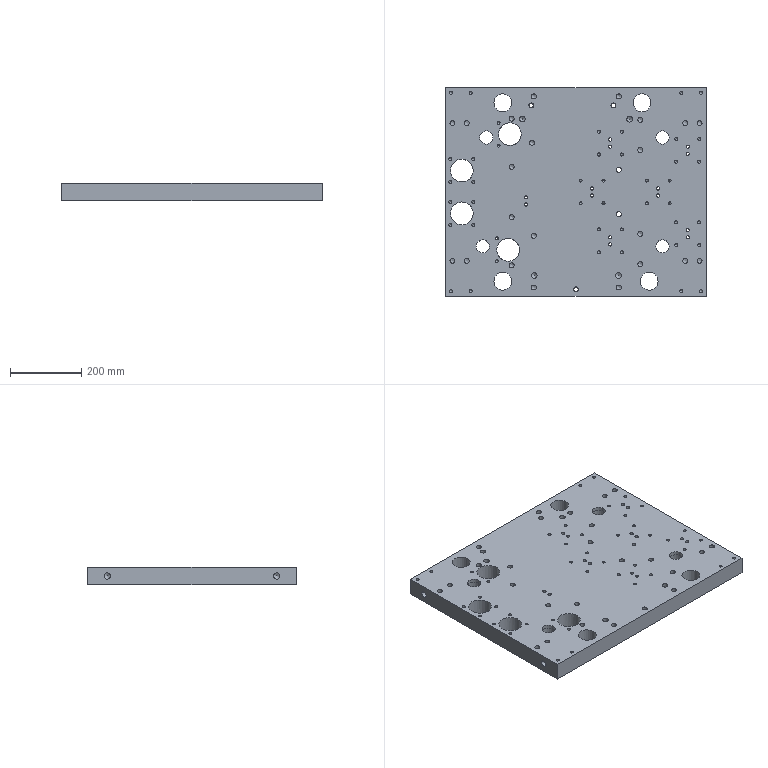Part | STEP file | PN_0001_id1150_x_t | 1 solid | 507 faces | box 730 x 585 x 50 mm | volume 18693036 mm3 | cylinder 250 | cone 197 | plane 36 | spline 24 | commonest cylinder face diameters 8.5 x112 14 x39 10 x22 9 x14 6.8 x13 5 x8